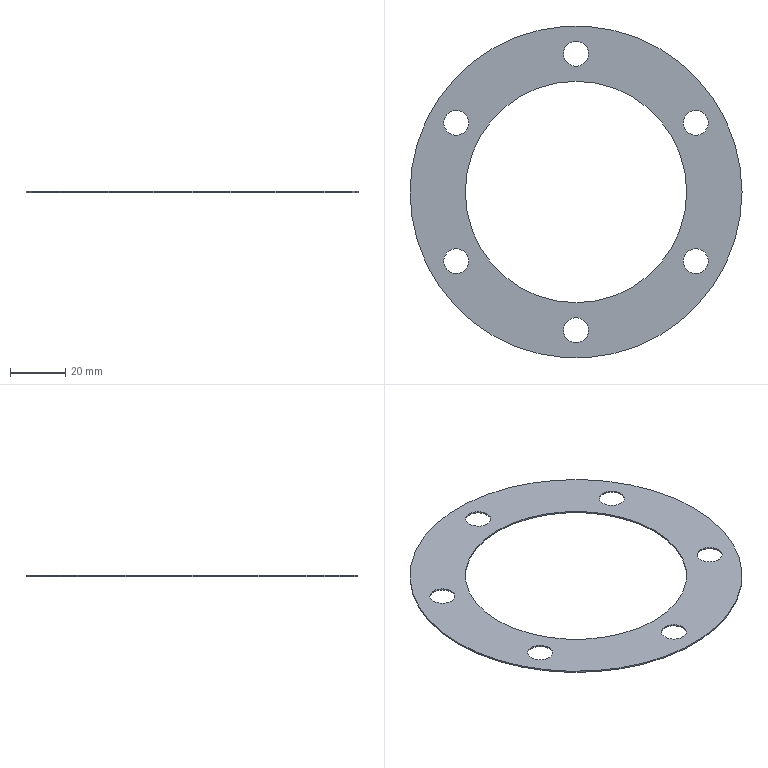Part | SolidWorks | features CirPattern 1, Extrusion 1, ICE 1 | 1 solid | 18 faces | box 120 x 120 x 0.5 mm | volume 2951 mm3 | cylinder 16 | plane 2 | commonest cylinder face diameters 9 x12 80 x2 120 x2
STEP:
#1=CARTESIAN_POINT('',(38.801,25.,0.));
#2=VERTEX_POINT('',#1);
#3=CARTESIAN_POINT('',(47.801,25.,0.));
#4=VERTEX_POINT('',#3);
#5=CARTESIAN_POINT('',(43.301,25.,0.));
#6=DIRECTION('',(0.,0.,1.));
#7=DIRECTION('',(0.5,-0.866,0.));
#8=AXIS2_PLACEMENT_3D('',#5,#6,#7);
#9=CIRCLE('',#8,4.5);
#10=EDGE_CURVE('',#2,#4,#9,.T.);
#11=ORIENTED_EDGE('',*,*,#10,.F.);
#12=CARTESIAN_POINT('',(38.801,25.,0.5));
#13=VERTEX_POINT('',#12);
#14=CARTESIAN_POINT('',(38.801,25.,0.));
#15=DIRECTION('',(0.,0.,1.));
#16=VECTOR('',#15,1000.);
#17=LINE('',#14,#16);
#18=EDGE_CURVE('',#2,#13,#17,.T.);
#19=ORIENTED_EDGE('',*,*,#18,.T.);
#20=CARTESIAN_POINT('',(47.801,25.,0.5));
#21=VERTEX_POINT('',#20);
#22=CARTESIAN_POINT('',(43.301,25.,0.5));
#23=DIRECTION('',(0.,0.,1.));
#24=DIRECTION('',(0.5,-0.866,0.));
#25=AXIS2_PLACEMENT_3D('',#22,#23,#24);
#26=CIRCLE('',#25,4.5);
#27=EDGE_CURVE('',#13,#21,#26,.T.);
#28=ORIENTED_EDGE('',*,*,#27,.T.);
#29=CARTESIAN_POINT('',(47.801,25.,0.));
#30=DIRECTION('',(0.,0.,1.));
#31=VECTOR('',#30,1000.);
#32=LINE('',#29,#31);
#33=EDGE_CURVE('',#4,#21,#32,.T.);
#34=ORIENTED_EDGE('',*,*,#33,.F.);
#35=EDGE_LOOP('',(#11,#19,#28,#34));
#36=FACE_OUTER_BOUND('',#35,.T.);
#37=CARTESIAN_POINT('',(43.301,25.,0.));
#38=DIRECTION('',(0.,0.,1.));
#39=DIRECTION('',(1.,0.,0.));
#40=AXIS2_PLACEMENT_3D('',#37,#38,#39);
#41=CYLINDRICAL_SURFACE('',#40,4.5);
#42=ADVANCED_FACE('',(#36),#41,.F.);
#43=CARTESIAN_POINT('',(38.801,-25.,0.));
#44=VERTEX_POINT('',#43);
#45=CARTESIAN_POINT('',(47.801,-25.,0.));
#46=VERTEX_POINT('',#45);
#47=CARTESIAN_POINT('',(43.301,-25.,0.));
#48=DIRECTION('',(0.,0.,1.));
#49=DIRECTION('',(-0.5,-0.866,0.));
#50=AXIS2_PLACEMENT_3D('',#47,#48,#49);
#51=CIRCLE('',#50,4.5);
#52=EDGE_CURVE('',#44,#46,#51,.T.);
#53=ORIENTED_EDGE('',*,*,#52,.F.);
#54=CARTESIAN_POINT('',(38.801,-25.,0.5));
#55=VERTEX_POINT('',#54);
#56=CARTESIAN_POINT('',(38.801,-25.,0.));
#57=DIRECTION('',(0.,0.,1.));
#58=VECTOR('',#57,1000.);
#59=LINE('',#56,#58);
#60=EDGE_CURVE('',#44,#55,#59,.T.);
#61=ORIENTED_EDGE('',*,*,#60,.T.);
#62=CARTESIAN_POINT('',(47.801,-25.,0.5));
#63=VERTEX_POINT('',#62);
#64=CARTESIAN_POINT('',(43.301,-25.,0.5));
#65=DIRECTION('',(0.,0.,1.));
#66=DIRECTION('',(-0.5,-0.866,0.));
#67=AXIS2_PLACEMENT_3D('',#64,#65,#66);
#68=CIRCLE('',#67,4.5);
#69=EDGE_CURVE('',#55,#63,#68,.T.);
#70=ORIENTED_EDGE('',*,*,#69,.T.);
#71=CARTESIAN_POINT('',(47.801,-25.,0.));
#72=DIRECTION('',(0.,0.,1.));
#73=VECTOR('',#72,1000.);
#74=LINE('',#71,#73);
#75=EDGE_CURVE('',#46,#63,#74,.T.);
#76=ORIENTED_EDGE('',*,*,#75,.F.);
#77=EDGE_LOOP('',(#53,#61,#70,#76));
#78=FACE_OUTER_BOUND('',#77,.T.);
#79=CARTESIAN_POINT('',(43.301,-25.,0.));
#80=DIRECTION('',(0.,0.,1.));
#81=DIRECTION('',(1.,0.,0.));
#82=AXIS2_PLACEMENT_3D('',#79,#80,#81);
#83=CYLINDRICAL_SURFACE('',#82,4.5);
#84=ADVANCED_FACE('',(#78),#83,.F.);
#85=CARTESIAN_POINT('',(-4.5,-50.,0.));
#86=VERTEX_POINT('',#85);
#87=CARTESIAN_POINT('',(4.5,-50.,0.));
#88=VERTEX_POINT('',#87);
#89=CARTESIAN_POINT('',(0.,-50.,0.));
#90=DIRECTION('',(0.,0.,1.));
#91=DIRECTION('',(-1.,0.,0.));
#92=AXIS2_PLACEMENT_3D('',#89,#90,#91);
#93=CIRCLE('',#92,4.5);
#94=EDGE_CURVE('',#86,#88,#93,.T.);
#95=ORIENTED_EDGE('',*,*,#94,.F.);
#96=CARTESIAN_POINT('',(-4.5,-50.,0.5));
#97=VERTEX_POINT('',#96);
#98=CARTESIAN_POINT('',(-4.5,-50.,0.));
#99=DIRECTION('',(0.,0.,1.));
#100=VECTOR('',#99,1000.);
#101=LINE('',#98,#100);
#102=EDGE_CURVE('',#86,#97,#101,.T.);
#103=ORIENTED_EDGE('',*,*,#102,.T.);
#104=CARTESIAN_POINT('',(4.5,-50.,0.5));
#105=VERTEX_POINT('',#104);
#106=CARTESIAN_POINT('',(0.,-50.,0.5));
#107=DIRECTION('',(0.,0.,1.));
#108=DIRECTION('',(-1.,0.,0.));
#109=AXIS2_PLACEMENT_3D('',#106,#107,#108);
#110=CIRCLE('',#109,4.5);
#111=EDGE_CURVE('',#97,#105,#110,.T.);
#112=ORIENTED_EDGE('',*,*,#111,.T.);
#113=CARTESIAN_POINT('',(4.5,-50.,0.));
#114=DIRECTION('',(0.,0.,1.));
#115=VECTOR('',#114,1000.);
#116=LINE('',#113,#115);
#117=EDGE_CURVE('',#88,#105,#116,.T.);
#118=ORIENTED_EDGE('',*,*,#117,.F.);
#119=EDGE_LOOP('',(#95,#103,#112,#118));
#120=FACE_OUTER_BOUND('',#119,.T.);
#121=CARTESIAN_POINT('',(0.,-50.,0.));
#122=DIRECTION('',(0.,0.,1.));
#123=DIRECTION('',(1.,0.,0.));
#124=AXIS2_PLACEMENT_3D('',#121,#122,#123);
#125=CYLINDRICAL_SURFACE('',#124,4.5);
#126=ADVANCED_FACE('',(#120),#125,.F.);
#127=CARTESIAN_POINT('',(-47.801,-25.,0.));
#128=VERTEX_POINT('',#127);
#129=CARTESIAN_POINT('',(-38.801,-25.,0.));
#130=VERTEX_POINT('',#129);
#131=CARTESIAN_POINT('',(-43.301,-25.,0.));
#132=DIRECTION('',(0.,0.,1.));
#133=DIRECTION('',(-0.5,0.866,0.));
#134=AXIS2_PLACEMENT_3D('',#131,#132,#133);
#135=CIRCLE('',#134,4.5);
#136=EDGE_CURVE('',#128,#130,#135,.T.);
#137=ORIENTED_EDGE('',*,*,#136,.F.);
#138=CARTESIAN_POINT('',(-47.801,-25.,0.5));
#139=VERTEX_POINT('',#138);
#140=CARTESIAN_POINT('',(-47.801,-25.,0.));
#141=DIRECTION('',(0.,0.,1.));
#142=VECTOR('',#141,1000.);
#143=LINE('',#140,#142);
#144=EDGE_CURVE('',#128,#139,#143,.T.);
#145=ORIENTED_EDGE('',*,*,#144,.T.);
#146=CARTESIAN_POINT('',(-38.801,-25.,0.5));
#147=VERTEX_POINT('',#146);
#148=CARTESIAN_POINT('',(-43.301,-25.,0.5));
#149=DIRECTION('',(0.,0.,1.));
#150=DIRECTION('',(-0.5,0.866,0.));
#151=AXIS2_PLACEMENT_3D('',#148,#149,#150);
#152=CIRCLE('',#151,4.5);
#153=EDGE_CURVE('',#139,#147,#152,.T.);
#154=ORIENTED_EDGE('',*,*,#153,.T.);
#155=CARTESIAN_POINT('',(-38.801,-25.,0.));
#156=DIRECTION('',(0.,0.,1.));
#157=VECTOR('',#156,1000.);
#158=LINE('',#155,#157);
#159=EDGE_CURVE('',#130,#147,#158,.T.);
#160=ORIENTED_EDGE('',*,*,#159,.F.);
#161=EDGE_LOOP('',(#137,#145,#154,#160));
#162=FACE_OUTER_BOUND('',#161,.T.);
#163=CARTESIAN_POINT('',(-43.301,-25.,0.));
#164=DIRECTION('',(0.,0.,1.));
#165=DIRECTION('',(1.,0.,0.));
#166=AXIS2_PLACEMENT_3D('',#163,#164,#165);
#167=CYLINDRICAL_SURFACE('',#166,4.5);
#168=ADVANCED_FACE('',(#162),#167,.F.);
#169=CARTESIAN_POINT('',(-47.801,25.,0.));
#170=VERTEX_POINT('',#169);
#171=CARTESIAN_POINT('',(-38.801,25.,0.));
#172=VERTEX_POINT('',#171);
#173=CARTESIAN_POINT('',(-43.301,25.,0.));
#174=DIRECTION('',(0.,0.,1.));
#175=DIRECTION('',(0.5,0.866,0.));
#176=AXIS2_PLACEMENT_3D('',#173,#174,#175);
#177=CIRCLE('',#176,4.5);
#178=EDGE_CURVE('',#170,#172,#177,.T.);
#179=ORIENTED_EDGE('',*,*,#178,.F.);
#180=CARTESIAN_POINT('',(-47.801,25.,0.5));
#181=VERTEX_POINT('',#180);
#182=CARTESIAN_POINT('',(-47.801,25.,0.));
#183=DIRECTION('',(0.,0.,1.));
#184=VECTOR('',#183,1000.);
#185=LINE('',#182,#184);
#186=EDGE_CURVE('',#170,#181,#185,.T.);
#187=ORIENTED_EDGE('',*,*,#186,.T.);
#188=CARTESIAN_POINT('',(-38.801,25.,0.5));
#189=VERTEX_POINT('',#188);
#190=CARTESIAN_POINT('',(-43.301,25.,0.5));
#191=DIRECTION('',(0.,0.,1.));
#192=DIRECTION('',(0.5,0.866,0.));
#193=AXIS2_PLACEMENT_3D('',#190,#191,#192);
#194=CIRCLE('',#193,4.5);
#195=EDGE_CURVE('',#181,#189,#194,.T.);
#196=ORIENTED_EDGE('',*,*,#195,.T.);
#197=CARTESIAN_POINT('',(-38.801,25.,0.));
#198=DIRECTION('',(0.,0.,1.));
#199=VECTOR('',#198,1000.);
#200=LINE('',#197,#199);
#201=EDGE_CURVE('',#172,#189,#200,.T.);
#202=ORIENTED_EDGE('',*,*,#201,.F.);
#203=EDGE_LOOP('',(#179,#187,#196,#202));
#204=FACE_OUTER_BOUND('',#203,.T.);
#205=CARTESIAN_POINT('',(-43.301,25.,0.));
#206=DIRECTION('',(0.,0.,1.));
#207=DIRECTION('',(1.,0.,0.));
#208=AXIS2_PLACEMENT_3D('',#205,#206,#207);
#209=CYLINDRICAL_SURFACE('',#208,4.5);
#210=ADVANCED_FACE('',(#204),#209,.F.);
#211=CARTESIAN_POINT('',(-4.5,50.,0.));
#212=VERTEX_POINT('',#211);
#213=CARTESIAN_POINT('',(4.5,50.,0.));
#214=VERTEX_POINT('',#213);
#215=CARTESIAN_POINT('',(0.,50.,0.));
#216=DIRECTION('',(0.,0.,1.));
#217=DIRECTION('',(1.,0.,0.));
#218=AXIS2_PLACEMENT_3D('',#215,#216,#217);
#219=CIRCLE('',#218,4.5);
#220=EDGE_CURVE('',#212,#214,#219,.T.);
#221=ORIENTED_EDGE('',*,*,#220,.F.);
#222=CARTESIAN_POINT('',(-4.5,50.,0.5));
#223=VERTEX_POINT('',#222);
#224=CARTESIAN_POINT('',(-4.5,50.,0.));
#225=DIRECTION('',(0.,0.,1.));
#226=VECTOR('',#225,1000.);
#227=LINE('',#224,#226);
#228=EDGE_CURVE('',#212,#223,#227,.T.);
#229=ORIENTED_EDGE('',*,*,#228,.T.);
#230=CARTESIAN_POINT('',(4.5,50.,0.5));
#231=VERTEX_POINT('',#230);
#232=CARTESIAN_POINT('',(0.,50.,0.5));
#233=DIRECTION('',(0.,0.,1.));
#234=DIRECTION('',(1.,0.,0.));
#235=AXIS2_PLACEMENT_3D('',#232,#233,#234);
#236=CIRCLE('',#235,4.5);
#237=EDGE_CURVE('',#223,#231,#236,.T.);
#238=ORIENTED_EDGE('',*,*,#237,.T.);
#239=CARTESIAN_POINT('',(4.5,50.,0.));
#240=DIRECTION('',(0.,0.,1.));
#241=VECTOR('',#240,1000.);
#242=LINE('',#239,#241);
#243=EDGE_CURVE('',#214,#231,#242,.T.);
#244=ORIENTED_EDGE('',*,*,#243,.F.);
#245=EDGE_LOOP('',(#221,#229,#238,#244));
#246=FACE_OUTER_BOUND('',#245,.T.);
#247=CARTESIAN_POINT('',(0.,50.,0.));
#248=DIRECTION('',(0.,0.,1.));
#249=DIRECTION('',(1.,0.,0.));
#250=AXIS2_PLACEMENT_3D('',#247,#248,#249);
#251=CYLINDRICAL_SURFACE('',#250,4.5);
#252=ADVANCED_FACE('',(#246),#251,.F.);
#253=CARTESIAN_POINT('',(-40.,0.,0.5));
#254=VERTEX_POINT('',#253);
#255=CARTESIAN_POINT('',(40.,0.,0.5));
#256=VERTEX_POINT('',#255);
#257=CARTESIAN_POINT('',(0.,0.,0.5));
#258=DIRECTION('',(0.,0.,1.));
#259=DIRECTION('',(1.,0.,0.));
#260=AXIS2_PLACEMENT_3D('',#257,#258,#259);
#261=CIRCLE('',#260,40.);
#262=EDGE_CURVE('',#254,#256,#261,.T.);
#263=ORIENTED_EDGE('',*,*,#262,.T.);
#264=CARTESIAN_POINT('',(40.,0.,0.));
#265=VERTEX_POINT('',#264);
#266=CARTESIAN_POINT('',(40.,0.,0.5));
#267=DIRECTION('',(0.,0.,-1.));
#268=VECTOR('',#267,1000.);
#269=LINE('',#266,#268);
#270=EDGE_CURVE('',#256,#265,#269,.T.);
#271=ORIENTED_EDGE('',*,*,#270,.T.);
#272=CARTESIAN_POINT('',(-40.,0.,0.));
#273=VERTEX_POINT('',#272);
#274=CARTESIAN_POINT('',(0.,0.,0.));
#275=DIRECTION('',(0.,0.,1.));
#276=DIRECTION('',(1.,0.,0.));
#277=AXIS2_PLACEMENT_3D('',#274,#275,#276);
#278=CIRCLE('',#277,40.);
#279=EDGE_CURVE('',#273,#265,#278,.T.);
#280=ORIENTED_EDGE('',*,*,#279,.F.);
#281=CARTESIAN_POINT('',(-40.,0.,0.5));
#282=DIRECTION('',(0.,0.,-1.));
#283=VECTOR('',#282,1000.);
#284=LINE('',#281,#283);
#285=EDGE_CURVE('',#254,#273,#284,.T.);
#286=ORIENTED_EDGE('',*,*,#285,.F.);
#287=EDGE_LOOP('',(#263,#271,#280,#286));
#288=FACE_OUTER_BOUND('',#287,.T.);
#289=CARTESIAN_POINT('',(0.,0.,0.5));
#290=DIRECTION('',(0.,0.,-1.));
#291=DIRECTION('',(-1.,0.,0.));
#292=AXIS2_PLACEMENT_3D('',#289,#290,#291);
#293=CYLINDRICAL_SURFACE('',#292,40.);
#294=ADVANCED_FACE('',(#288),#293,.F.);
#295=CARTESIAN_POINT('',(60.,0.,0.5));
#296=VERTEX_POINT('',#295);
#297=CARTESIAN_POINT('',(-60.,0.,0.5));
#298=VERTEX_POINT('',#297);
#299=CARTESIAN_POINT('',(0.,0.,0.5));
#300=DIRECTION('',(0.,0.,1.));
#301=DIRECTION('',(1.,0.,0.));
#302=AXIS2_PLACEMENT_3D('',#299,#300,#301);
#303=CIRCLE('',#302,60.);
#304=EDGE_CURVE('',#296,#298,#303,.T.);
#305=ORIENTED_EDGE('',*,*,#304,.F.);
#306=CARTESIAN_POINT('',(60.,0.,0.));
#307=VERTEX_POINT('',#306);
#308=CARTESIAN_POINT('',(60.,0.,0.5));
#309=DIRECTION('',(0.,0.,-1.));
#310=VECTOR('',#309,1000.);
#311=LINE('',#308,#310);
#312=EDGE_CURVE('',#296,#307,#311,.T.);
#313=ORIENTED_EDGE('',*,*,#312,.T.);
#314=CARTESIAN_POINT('',(-60.,0.,0.));
#315=VERTEX_POINT('',#314);
#316=CARTESIAN_POINT('',(0.,0.,0.));
#317=DIRECTION('',(0.,0.,1.));
#318=DIRECTION('',(1.,0.,0.));
#319=AXIS2_PLACEMENT_3D('',#316,#317,#318);
#320=CIRCLE('',#319,60.);
#321=EDGE_CURVE('',#307,#315,#320,.T.);
#322=ORIENTED_EDGE('',*,*,#321,.T.);
#323=CARTESIAN_POINT('',(-60.,0.,0.5));
#324=DIRECTION('',(0.,0.,-1.));
#325=VECTOR('',#324,1000.);
#326=LINE('',#323,#325);
#327=EDGE_CURVE('',#298,#315,#326,.T.);
#328=ORIENTED_EDGE('',*,*,#327,.F.);
#329=EDGE_LOOP('',(#305,#313,#322,#328));
#330=FACE_OUTER_BOUND('',#329,.T.);
#331=CARTESIAN_POINT('',(0.,0.,0.5));
#332=DIRECTION('',(0.,0.,-1.));
#333=DIRECTION('',(-1.,0.,0.));
#334=AXIS2_PLACEMENT_3D('',#331,#332,#333);
#335=CYLINDRICAL_SURFACE('',#334,60.);
#336=ADVANCED_FACE('',(#330),#335,.T.);
#337=CARTESIAN_POINT('',(43.301,25.,0.5));
#338=DIRECTION('',(0.,0.,1.));
#339=DIRECTION('',(0.5,-0.866,0.));
#340=AXIS2_PLACEMENT_3D('',#337,#338,#339);
#341=CIRCLE('',#340,4.5);
#342=EDGE_CURVE('',#21,#13,#341,.T.);
#343=ORIENTED_EDGE('',*,*,#342,.F.);
#344=ORIENTED_EDGE('',*,*,#27,.F.);
#345=EDGE_LOOP('',(#343,#344));
#346=FACE_BOUND('',#345,.T.);
#347=CARTESIAN_POINT('',(43.301,-25.,0.5));
#348=DIRECTION('',(0.,0.,1.));
#349=DIRECTION('',(-0.5,-0.866,0.));
#350=AXIS2_PLACEMENT_3D('',#347,#348,#349);
#351=CIRCLE('',#350,4.5);
#352=EDGE_CURVE('',#63,#55,#351,.T.);
#353=ORIENTED_EDGE('',*,*,#352,.F.);
#354=ORIENTED_EDGE('',*,*,#69,.F.);
#355=EDGE_LOOP('',(#353,#354));
#356=FACE_BOUND('',#355,.T.);
#357=CARTESIAN_POINT('',(0.,-50.,0.5));
#358=DIRECTION('',(0.,0.,1.));
#359=DIRECTION('',(-1.,0.,0.));
#360=AXIS2_PLACEMENT_3D('',#357,#358,#359);
#361=CIRCLE('',#360,4.5);
#362=EDGE_CURVE('',#105,#97,#361,.T.);
#363=ORIENTED_EDGE('',*,*,#362,.F.);
#364=ORIENTED_EDGE('',*,*,#111,.F.);
#365=EDGE_LOOP('',(#363,#364));
#366=FACE_BOUND('',#365,.T.);
#367=CARTESIAN_POINT('',(-43.301,-25.,0.5));
#368=DIRECTION('',(0.,0.,1.));
#369=DIRECTION('',(-0.5,0.866,0.));
#370=AXIS2_PLACEMENT_3D('',#367,#368,#369);
#371=CIRCLE('',#370,4.5);
#372=EDGE_CURVE('',#147,#139,#371,.T.);
#373=ORIENTED_EDGE('',*,*,#372,.F.);
#374=ORIENTED_EDGE('',*,*,#153,.F.);
#375=EDGE_LOOP('',(#373,#374));
#376=FACE_BOUND('',#375,.T.);
#377=CARTESIAN_POINT('',(-43.301,25.,0.5));
#378=DIRECTION('',(0.,0.,1.));
#379=DIRECTION('',(0.5,0.866,0.));
#380=AXIS2_PLACEMENT_3D('',#377,#378,#379);
#381=CIRCLE('',#380,4.5);
#382=EDGE_CURVE('',#189,#181,#381,.T.);
#383=ORIENTED_EDGE('',*,*,#382,.F.);
#384=ORIENTED_EDGE('',*,*,#195,.F.);
#385=EDGE_LOOP('',(#383,#384));
#386=FACE_BOUND('',#385,.T.);
#387=CARTESIAN_POINT('',(0.,50.,0.5));
#388=DIRECTION('',(0.,0.,1.));
#389=DIRECTION('',(1.,0.,0.));
#390=AXIS2_PLACEMENT_3D('',#387,#388,#389);
#391=CIRCLE('',#390,4.5);
#392=EDGE_CURVE('',#231,#223,#391,.T.);
#393=ORIENTED_EDGE('',*,*,#392,.F.);
#394=ORIENTED_EDGE('',*,*,#237,.F.);
#395=EDGE_LOOP('',(#393,#394));
#396=FACE_BOUND('',#395,.T.);
#397=CARTESIAN_POINT('',(0.,0.,0.5));
#398=DIRECTION('',(0.,0.,1.));
#399=DIRECTION('',(1.,0.,0.));
#400=AXIS2_PLACEMENT_3D('',#397,#398,#399);
#401=CIRCLE('',#400,60.);
#402=EDGE_CURVE('',#298,#296,#401,.T.);
#403=ORIENTED_EDGE('',*,*,#402,.T.);
#404=ORIENTED_EDGE('',*,*,#304,.T.);
#405=EDGE_LOOP('',(#403,#404));
#406=FACE_OUTER_BOUND('',#405,.T.);
#407=ORIENTED_EDGE('',*,*,#262,.F.);
#408=CARTESIAN_POINT('',(0.,0.,0.5));
#409=DIRECTION('',(0.,0.,1.));
#410=DIRECTION('',(1.,0.,0.));
#411=AXIS2_PLACEMENT_3D('',#408,#409,#410);
#412=CIRCLE('',#411,40.);
#413=EDGE_CURVE('',#256,#254,#412,.T.);
#414=ORIENTED_EDGE('',*,*,#413,.F.);
#415=EDGE_LOOP('',(#407,#414));
#416=FACE_BOUND('',#415,.T.);
#417=CARTESIAN_POINT('',(0.,0.,0.5));
#418=DIRECTION('',(0.,0.,1.));
#419=DIRECTION('',(1.,0.,0.));
#420=AXIS2_PLACEMENT_3D('',#417,#418,#419);
#421=PLANE('',#420);
#422=ADVANCED_FACE('',(#346,#356,#366,#376,#386,#396,#406,#416),#421,.T.);
#423=CARTESIAN_POINT('',(43.301,25.,0.));
#424=DIRECTION('',(0.,0.,1.));
#425=DIRECTION('',(0.5,-0.866,0.));
#426=AXIS2_PLACEMENT_3D('',#423,#424,#425);
#427=CIRCLE('',#426,4.5);
#428=EDGE_CURVE('',#4,#2,#427,.T.);
#429=ORIENTED_EDGE('',*,*,#428,.T.);
#430=ORIENTED_EDGE('',*,*,#10,.T.);
#431=EDGE_LOOP('',(#429,#430));
#432=FACE_BOUND('',#431,.T.);
#433=CARTESIAN_POINT('',(43.301,-25.,0.));
#434=DIRECTION('',(0.,0.,1.));
#435=DIRECTION('',(-0.5,-0.866,0.));
#436=AXIS2_PLACEMENT_3D('',#433,#434,#435);
#437=CIRCLE('',#436,4.5);
#438=EDGE_CURVE('',#46,#44,#437,.T.);
#439=ORIENTED_EDGE('',*,*,#438,.T.);
#440=ORIENTED_EDGE('',*,*,#52,.T.);
#441=EDGE_LOOP('',(#439,#440));
#442=FACE_BOUND('',#441,.T.);
#443=CARTESIAN_POINT('',(0.,-50.,0.));
#444=DIRECTION('',(0.,0.,1.));
#445=DIRECTION('',(-1.,0.,0.));
#446=AXIS2_PLACEMENT_3D('',#443,#444,#445);
#447=CIRCLE('',#446,4.5);
#448=EDGE_CURVE('',#88,#86,#447,.T.);
#449=ORIENTED_EDGE('',*,*,#448,.T.);
#450=ORIENTED_EDGE('',*,*,#94,.T.);
#451=EDGE_LOOP('',(#449,#450));
#452=FACE_BOUND('',#451,.T.);
#453=CARTESIAN_POINT('',(-43.301,-25.,0.));
#454=DIRECTION('',(0.,0.,1.));
#455=DIRECTION('',(-0.5,0.866,0.));
#456=AXIS2_PLACEMENT_3D('',#453,#454,#455);
#457=CIRCLE('',#456,4.5);
#458=EDGE_CURVE('',#130,#128,#457,.T.);
#459=ORIENTED_EDGE('',*,*,#458,.T.);
#460=ORIENTED_EDGE('',*,*,#136,.T.);
#461=EDGE_LOOP('',(#459,#460));
#462=FACE_BOUND('',#461,.T.);
#463=CARTESIAN_POINT('',(-43.301,25.,0.));
#464=DIRECTION('',(0.,0.,1.));
#465=DIRECTION('',(0.5,0.866,0.));
#466=AXIS2_PLACEMENT_3D('',#463,#464,#465);
#467=CIRCLE('',#466,4.5);
#468=EDGE_CURVE('',#172,#170,#467,.T.);
#469=ORIENTED_EDGE('',*,*,#468,.T.);
#470=ORIENTED_EDGE('',*,*,#178,.T.);
#471=EDGE_LOOP('',(#469,#470));
#472=FACE_BOUND('',#471,.T.);
#473=CARTESIAN_POINT('',(0.,50.,0.));
#474=DIRECTION('',(0.,0.,1.));
#475=DIRECTION('',(1.,0.,0.));
#476=AXIS2_PLACEMENT_3D('',#473,#474,#475);
#477=CIRCLE('',#476,4.5);
#478=EDGE_CURVE('',#214,#212,#477,.T.);
#479=ORIENTED_EDGE('',*,*,#478,.T.);
#480=ORIENTED_EDGE('',*,*,#220,.T.);
#481=EDGE_LOOP('',(#479,#480));
#482=FACE_BOUND('',#481,.T.);
#483=CARTESIAN_POINT('',(0.,0.,0.));
#484=DIRECTION('',(0.,0.,1.));
#485=DIRECTION('',(1.,0.,0.));
#486=AXIS2_PLACEMENT_3D('',#483,#484,#485);
#487=CIRCLE('',#486,60.);
#488=EDGE_CURVE('',#315,#307,#487,.T.);
#489=ORIENTED_EDGE('',*,*,#488,.F.);
#490=ORIENTED_EDGE('',*,*,#321,.F.);
#491=EDGE_LOOP('',(#489,#490));
#492=FACE_OUTER_BOUND('',#491,.T.);
#493=ORIENTED_EDGE('',*,*,#279,.T.);
#494=CARTESIAN_POINT('',(0.,0.,0.));
#495=DIRECTION('',(0.,0.,1.));
#496=DIRECTION('',(1.,0.,0.));
#497=AXIS2_PLACEMENT_3D('',#494,#495,#496);
#498=CIRCLE('',#497,40.);
#499=EDGE_CURVE('',#265,#273,#498,.T.);
#500=ORIENTED_EDGE('',*,*,#499,.T.);
#501=EDGE_LOOP('',(#493,#500));
#502=FACE_BOUND('',#501,.T.);
#503=CARTESIAN_POINT('',(0.,0.,0.));
#504=DIRECTION('',(0.,0.,1.));
#505=DIRECTION('',(1.,0.,0.));
#506=AXIS2_PLACEMENT_3D('',#503,#504,#505);
#507=PLANE('',#506);
#508=ADVANCED_FACE('',(#432,#442,#452,#462,#472,#482,#492,#502),#507,.F.);
#509=ORIENTED_EDGE('',*,*,#312,.F.);
#510=ORIENTED_EDGE('',*,*,#402,.F.);
#511=ORIENTED_EDGE('',*,*,#327,.T.);
#512=ORIENTED_EDGE('',*,*,#488,.T.);
#513=EDGE_LOOP('',(#509,#510,#511,#512));
#514=FACE_OUTER_BOUND('',#513,.T.);
#515=CARTESIAN_POINT('',(0.,0.,0.5));
#516=DIRECTION('',(0.,0.,-1.));
#517=DIRECTION('',(-1.,0.,0.));
#518=AXIS2_PLACEMENT_3D('',#515,#516,#517);
#519=CYLINDRICAL_SURFACE('',#518,60.);
#520=ADVANCED_FACE('',(#514),#519,.T.);
#521=ORIENTED_EDGE('',*,*,#270,.F.);
#522=ORIENTED_EDGE('',*,*,#413,.T.);
#523=ORIENTED_EDGE('',*,*,#285,.T.);
#524=ORIENTED_EDGE('',*,*,#499,.F.);
#525=EDGE_LOOP('',(#521,#522,#523,#524));
#526=FACE_OUTER_BOUND('',#525,.T.);
#527=CARTESIAN_POINT('',(0.,0.,0.5));
#528=DIRECTION('',(0.,0.,-1.));
#529=DIRECTION('',(-1.,0.,0.));
#530=AXIS2_PLACEMENT_3D('',#527,#528,#529);
#531=CYLINDRICAL_SURFACE('',#530,40.);
#532=ADVANCED_FACE('',(#526),#531,.F.);
#533=ORIENTED_EDGE('',*,*,#228,.F.);
#534=ORIENTED_EDGE('',*,*,#478,.F.);
#535=ORIENTED_EDGE('',*,*,#243,.T.);
#536=ORIENTED_EDGE('',*,*,#392,.T.);
#537=EDGE_LOOP('',(#533,#534,#535,#536));
#538=FACE_OUTER_BOUND('',#537,.T.);
#539=CARTESIAN_POINT('',(0.,50.,0.));
#540=DIRECTION('',(0.,0.,1.));
#541=DIRECTION('',(1.,0.,0.));
#542=AXIS2_PLACEMENT_3D('',#539,#540,#541);
#543=CYLINDRICAL_SURFACE('',#542,4.5);
#544=ADVANCED_FACE('',(#538),#543,.F.);
#545=ORIENTED_EDGE('',*,*,#186,.F.);
#546=ORIENTED_EDGE('',*,*,#468,.F.);
#547=ORIENTED_EDGE('',*,*,#201,.T.);
#548=ORIENTED_EDGE('',*,*,#382,.T.);
#549=EDGE_LOOP('',(#545,#546,#547,#548));
#550=FACE_OUTER_BOUND('',#549,.T.);
#551=CARTESIAN_POINT('',(-43.301,25.,0.));
#552=DIRECTION('',(0.,0.,1.));
#553=DIRECTION('',(1.,0.,0.));
#554=AXIS2_PLACEMENT_3D('',#551,#552,#553);
#555=CYLINDRICAL_SURFACE('',#554,4.5);
#556=ADVANCED_FACE('',(#550),#555,.F.);
#557=ORIENTED_EDGE('',*,*,#144,.F.);
#558=ORIENTED_EDGE('',*,*,#458,.F.);
#559=ORIENTED_EDGE('',*,*,#159,.T.);
#560=ORIENTED_EDGE('',*,*,#372,.T.);
#561=EDGE_LOOP('',(#557,#558,#559,#560));
#562=FACE_OUTER_BOUND('',#561,.T.);
#563=CARTESIAN_POINT('',(-43.301,-25.,0.));
#564=DIRECTION('',(0.,0.,1.));
#565=DIRECTION('',(1.,0.,0.));
#566=AXIS2_PLACEMENT_3D('',#563,#564,#565);
#567=CYLINDRICAL_SURFACE('',#566,4.5);
#568=ADVANCED_FACE('',(#562),#567,.F.);
#569=ORIENTED_EDGE('',*,*,#102,.F.);
#570=ORIENTED_EDGE('',*,*,#448,.F.);
#571=ORIENTED_EDGE('',*,*,#117,.T.);
#572=ORIENTED_EDGE('',*,*,#362,.T.);
#573=EDGE_LOOP('',(#569,#570,#571,#572));
#574=FACE_OUTER_BOUND('',#573,.T.);
#575=CARTESIAN_POINT('',(0.,-50.,0.));
#576=DIRECTION('',(0.,0.,1.));
#577=DIRECTION('',(1.,0.,0.));
#578=AXIS2_PLACEMENT_3D('',#575,#576,#577);
#579=CYLINDRICAL_SURFACE('',#578,4.5);
#580=ADVANCED_FACE('',(#574),#579,.F.);
#581=ORIENTED_EDGE('',*,*,#60,.F.);
#582=ORIENTED_EDGE('',*,*,#438,.F.);
#583=ORIENTED_EDGE('',*,*,#75,.T.);
#584=ORIENTED_EDGE('',*,*,#352,.T.);
#585=EDGE_LOOP('',(#581,#582,#583,#584));
#586=FACE_OUTER_BOUND('',#585,.T.);
#587=CARTESIAN_POINT('',(43.301,-25.,0.));
#588=DIRECTION('',(0.,0.,1.));
#589=DIRECTION('',(1.,0.,0.));
#590=AXIS2_PLACEMENT_3D('',#587,#588,#589);
#591=CYLINDRICAL_SURFACE('',#590,4.5);
#592=ADVANCED_FACE('',(#586),#591,.F.);
#593=ORIENTED_EDGE('',*,*,#18,.F.);
#594=ORIENTED_EDGE('',*,*,#428,.F.);
#595=ORIENTED_EDGE('',*,*,#33,.T.);
#596=ORIENTED_EDGE('',*,*,#342,.T.);
#597=EDGE_LOOP('',(#593,#594,#595,#596));
#598=FACE_OUTER_BOUND('',#597,.T.);
#599=CARTESIAN_POINT('',(43.301,25.,0.));
#600=DIRECTION('',(0.,0.,1.));
#601=DIRECTION('',(1.,0.,0.));
#602=AXIS2_PLACEMENT_3D('',#599,#600,#601);
#603=CYLINDRICAL_SURFACE('',#602,4.5);
#604=ADVANCED_FACE('',(#598),#603,.F.);
#605=CLOSED_SHELL('',(#42,#84,#126,#168,#210,#252,#294,#336,#422,#508,#520,#532,#544,#556,#568,#580,#592,#604));
#606=MANIFOLD_SOLID_BREP('',#605);
#607=CARTESIAN_POINT('',(0.,0.,0.));
#608=DIRECTION('',(0.,0.,1.));
#609=DIRECTION('',(1.,0.,0.));
#610=AXIS2_PLACEMENT_3D('',#607,#608,#609);
#611=(LENGTH_UNIT()NAMED_UNIT(*)SI_UNIT(.MILLI.,.METRE.));
#612=UNCERTAINTY_MEASURE_WITH_UNIT(LENGTH_MEASURE(0.00001),#611,'','');
#613=(NAMED_UNIT(*)PLANE_ANGLE_UNIT()SI_UNIT($,.RADIAN.));
#614=(NAMED_UNIT(*)SI_UNIT($,.STERADIAN.)SOLID_ANGLE_UNIT());
#615=(GEOMETRIC_REPRESENTATION_CONTEXT(3)GLOBAL_UNCERTAINTY_ASSIGNED_CONTEXT((#612))GLOBAL_UNIT_ASSIGNED_CONTEXT((#611,#613,#614))REPRESENTATION_CONTEXT('',''));
#616=ADVANCED_BREP_SHAPE_REPRESENTATION('',(#606,#610),#615);